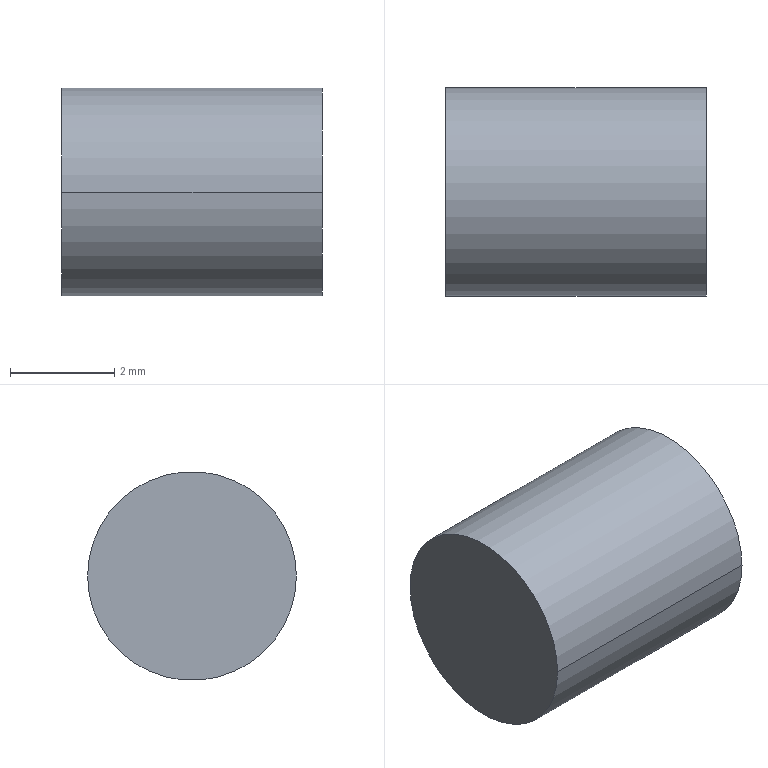Part | NX | 1 solid | 4 faces | box 5 x 4 x 4 mm | volume 62.832 mm3 | cylinder 2 | plane 2 | commonest cylinder face diameters 4 x2
STEP:
#1=CARTESIAN_POINT('',(-63.,168.376,-94.516));
#2=VERTEX_POINT('',#1);
#3=CARTESIAN_POINT('',(-63.,164.376,-94.516));
#4=VERTEX_POINT('',#3);
#5=CARTESIAN_POINT('',(-63.,166.376,-94.516));
#6=DIRECTION('',(-1.,0.,0.));
#7=DIRECTION('',(0.,-1.,0.));
#8=AXIS2_PLACEMENT_3D('',#5,#6,#7);
#9=CIRCLE('',#8,2.);
#10=EDGE_CURVE('',#2,#4,#9,.T.);
#11=ORIENTED_EDGE('',*,*,#10,.T.);
#12=CARTESIAN_POINT('',(-68.,164.376,-94.516));
#13=VERTEX_POINT('',#12);
#14=CARTESIAN_POINT('',(-68.,164.376,-94.516));
#15=DIRECTION('',(-1.,0.,0.));
#16=VECTOR('',#15,1000.);
#17=LINE('',#14,#16);
#18=EDGE_CURVE('',#13,#4,#17,.F.);
#19=ORIENTED_EDGE('',*,*,#18,.F.);
#20=CARTESIAN_POINT('',(-68.,168.376,-94.516));
#21=VERTEX_POINT('',#20);
#22=CARTESIAN_POINT('',(-68.,166.376,-94.516));
#23=DIRECTION('',(-1.,0.,0.));
#24=DIRECTION('',(0.,-1.,0.));
#25=AXIS2_PLACEMENT_3D('',#22,#23,#24);
#26=CIRCLE('',#25,2.);
#27=EDGE_CURVE('',#21,#13,#26,.T.);
#28=ORIENTED_EDGE('',*,*,#27,.F.);
#29=CARTESIAN_POINT('',(-68.,168.376,-94.516));
#30=DIRECTION('',(-1.,0.,0.));
#31=VECTOR('',#30,1000.);
#32=LINE('',#29,#31);
#33=EDGE_CURVE('',#21,#2,#32,.F.);
#34=ORIENTED_EDGE('',*,*,#33,.T.);
#35=EDGE_LOOP('',(#11,#19,#28,#34));
#36=FACE_BOUND('',#35,.T.);
#37=CARTESIAN_POINT('',(-68.,166.376,-94.516));
#38=DIRECTION('',(-1.,0.,0.));
#39=DIRECTION('',(0.,-1.,0.));
#40=AXIS2_PLACEMENT_3D('',#37,#38,#39);
#41=CYLINDRICAL_SURFACE('',#40,2.);
#42=ADVANCED_FACE('',(#36),#41,.T.);
#43=ORIENTED_EDGE('',*,*,#18,.T.);
#44=CARTESIAN_POINT('',(-63.,166.376,-94.516));
#45=DIRECTION('',(-1.,0.,0.));
#46=DIRECTION('',(0.,-1.,0.));
#47=AXIS2_PLACEMENT_3D('',#44,#45,#46);
#48=CIRCLE('',#47,2.);
#49=EDGE_CURVE('',#4,#2,#48,.T.);
#50=ORIENTED_EDGE('',*,*,#49,.T.);
#51=ORIENTED_EDGE('',*,*,#33,.F.);
#52=CARTESIAN_POINT('',(-68.,166.376,-94.516));
#53=DIRECTION('',(-1.,0.,0.));
#54=DIRECTION('',(0.,-1.,0.));
#55=AXIS2_PLACEMENT_3D('',#52,#53,#54);
#56=CIRCLE('',#55,2.);
#57=EDGE_CURVE('',#13,#21,#56,.T.);
#58=ORIENTED_EDGE('',*,*,#57,.F.);
#59=EDGE_LOOP('',(#43,#50,#51,#58));
#60=FACE_BOUND('',#59,.T.);
#61=CARTESIAN_POINT('',(-68.,166.376,-94.516));
#62=DIRECTION('',(-1.,0.,0.));
#63=DIRECTION('',(0.,-1.,0.));
#64=AXIS2_PLACEMENT_3D('',#61,#62,#63);
#65=CYLINDRICAL_SURFACE('',#64,2.);
#66=ADVANCED_FACE('',(#60),#65,.T.);
#67=ORIENTED_EDGE('',*,*,#10,.F.);
#68=ORIENTED_EDGE('',*,*,#49,.F.);
#69=EDGE_LOOP('',(#67,#68));
#70=FACE_BOUND('',#69,.T.);
#71=CARTESIAN_POINT('',(-63.,166.053,-93.037));
#72=DIRECTION('',(1.,0.,0.));
#73=DIRECTION('',(0.,-1.,0.));
#74=AXIS2_PLACEMENT_3D('',#71,#72,#73);
#75=PLANE('',#74);
#76=ADVANCED_FACE('',(#70),#75,.T.);
#77=ORIENTED_EDGE('',*,*,#27,.T.);
#78=ORIENTED_EDGE('',*,*,#57,.T.);
#79=EDGE_LOOP('',(#77,#78));
#80=FACE_BOUND('',#79,.T.);
#81=CARTESIAN_POINT('',(-68.,166.053,-93.037));
#82=DIRECTION('',(1.,0.,0.));
#83=DIRECTION('',(0.,-1.,0.));
#84=AXIS2_PLACEMENT_3D('',#81,#82,#83);
#85=PLANE('',#84);
#86=ADVANCED_FACE('',(#80),#85,.F.);
#87=CLOSED_SHELL('',(#42,#66,#76,#86));
#88=MANIFOLD_SOLID_BREP('',#87);
#89=(LENGTH_UNIT()NAMED_UNIT(*)SI_UNIT(.MILLI.,.METRE.));
#90=UNCERTAINTY_MEASURE_WITH_UNIT(LENGTH_MEASURE(0.00001),#89,'','');
#91=(NAMED_UNIT(*)PLANE_ANGLE_UNIT()SI_UNIT($,.RADIAN.));
#92=(NAMED_UNIT(*)SI_UNIT($,.STERADIAN.)SOLID_ANGLE_UNIT());
#93=(GEOMETRIC_REPRESENTATION_CONTEXT(3)GLOBAL_UNCERTAINTY_ASSIGNED_CONTEXT((#90))GLOBAL_UNIT_ASSIGNED_CONTEXT((#89,#91,#92))REPRESENTATION_CONTEXT('',''));
#94=ADVANCED_BREP_SHAPE_REPRESENTATION('',(#88),#93);